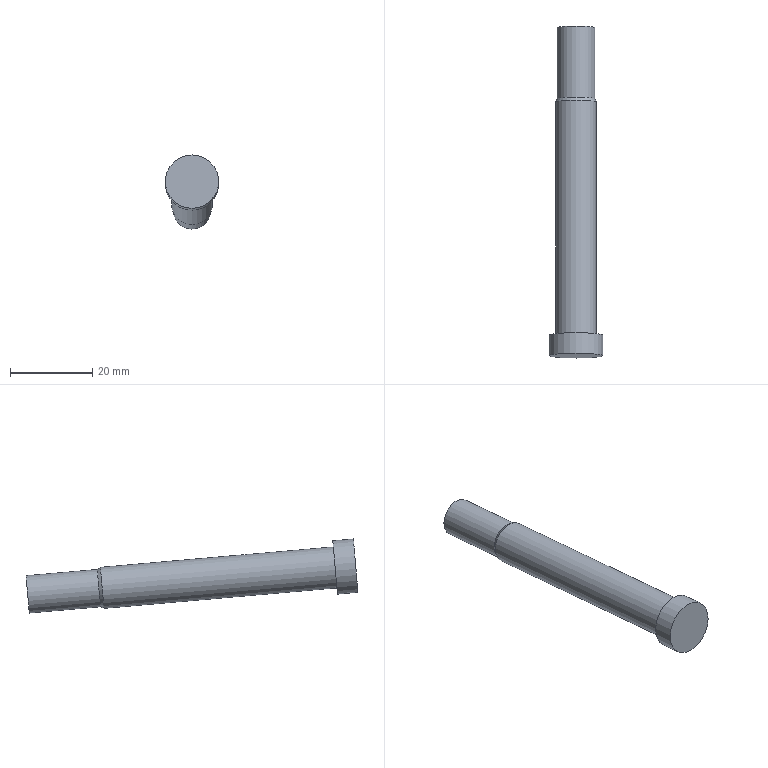Part | NX | features SPAS 10-80-7.100 2 | 1 solid | 7 faces | box 13 x 80.659 x 17.98 mm | volume 6314 mm3 | plane 3 | cylinder 3 | torus 1 | commonest cylinder face diameters 9.1 x1 10 x1 13 x1
STEP:
#1=CARTESIAN_POINT('',(-561.105,-62.517,-39.823));
#2=VERTEX_POINT('',#1);
#3=CARTESIAN_POINT('',(-561.105,-62.913,-44.355));
#4=DIRECTION('',(0.,0.9962,-0.08716));
#5=DIRECTION('',(0.,0.08716,0.9962));
#6=AXIS2_PLACEMENT_3D('',#3,#4,#5);
#7=CIRCLE('',#6,4.55);
#8=EDGE_CURVE('',#2,#2,#7,.F.);
#9=ORIENTED_EDGE('',*,*,#8,.F.);
#10=EDGE_LOOP('',(#9));
#11=FACE_BOUND('',#10,.T.);
#12=CARTESIAN_POINT('',(-561.105,-62.913,-44.355));
#13=DIRECTION('',(0.,0.9962,-0.08716));
#14=DIRECTION('',(0.,0.08716,0.9962));
#15=AXIS2_PLACEMENT_3D('',#12,#13,#14);
#16=PLANE('',#15);
#17=ADVANCED_FACE('',(#11),#16,.T.);
#18=CARTESIAN_POINT('',(-561.105,-79.809,-38.31));
#19=VERTEX_POINT('',#18);
#20=CARTESIAN_POINT('',(-561.105,-80.206,-42.843));
#21=DIRECTION('',(0.,0.9962,-0.08716));
#22=DIRECTION('',(0.,0.08716,0.9962));
#23=AXIS2_PLACEMENT_3D('',#20,#21,#22);
#24=CIRCLE('',#23,4.55);
#25=EDGE_CURVE('',#19,#19,#24,.T.);
#26=ORIENTED_EDGE('',*,*,#25,.T.);
#27=EDGE_LOOP('',(#26));
#28=FACE_BOUND('',#27,.T.);
#29=ORIENTED_EDGE('',*,*,#8,.T.);
#30=EDGE_LOOP('',(#29));
#31=FACE_BOUND('',#30,.T.);
#32=CARTESIAN_POINT('',(-561.105,-62.913,-44.355));
#33=DIRECTION('',(0.,-0.9962,0.08716));
#34=DIRECTION('',(0.,-0.08716,-0.9962));
#35=AXIS2_PLACEMENT_3D('',#32,#33,#34);
#36=CYLINDRICAL_SURFACE('',#35,4.55);
#37=ADVANCED_FACE('',(#28,#31),#36,.T.);
#38=CARTESIAN_POINT('',(-561.105,-137.192,-32.838));
#39=VERTEX_POINT('',#38);
#40=CARTESIAN_POINT('',(-561.105,-137.628,-37.819));
#41=DIRECTION('',(0.,0.9962,-0.08716));
#42=DIRECTION('',(0.,0.08716,0.9962));
#43=AXIS2_PLACEMENT_3D('',#40,#41,#42);
#44=CIRCLE('',#43,5.);
#45=EDGE_CURVE('',#39,#39,#44,.F.);
#46=ORIENTED_EDGE('',*,*,#45,.F.);
#47=EDGE_LOOP('',(#46));
#48=FACE_BOUND('',#47,.T.);
#49=CARTESIAN_POINT('',(-561.105,-81.466,-47.751));
#50=VERTEX_POINT('',#49);
#51=CARTESIAN_POINT('',(-561.105,-81.03,-42.77));
#52=DIRECTION('',(0.,-0.9962,0.08716));
#53=DIRECTION('',(0.,-0.08716,-0.9962));
#54=AXIS2_PLACEMENT_3D('',#51,#52,#53);
#55=CIRCLE('',#54,5.);
#56=EDGE_CURVE('',#50,#50,#55,.T.);
#57=ORIENTED_EDGE('',*,*,#56,.T.);
#58=EDGE_LOOP('',(#57));
#59=FACE_BOUND('',#58,.T.);
#60=CARTESIAN_POINT('',(-561.105,-81.03,-42.77));
#61=DIRECTION('',(0.,-0.9962,0.08716));
#62=DIRECTION('',(0.,-0.08716,-0.9962));
#63=AXIS2_PLACEMENT_3D('',#60,#61,#62);
#64=CYLINDRICAL_SURFACE('',#63,5.);
#65=ADVANCED_FACE('',(#48,#59),#64,.T.);
#66=CARTESIAN_POINT('',(-561.105,-142.042,-30.908));
#67=VERTEX_POINT('',#66);
#68=CARTESIAN_POINT('',(-561.105,-142.609,-37.383));
#69=DIRECTION('',(0.,0.9962,-0.08716));
#70=DIRECTION('',(0.,0.08716,0.9962));
#71=AXIS2_PLACEMENT_3D('',#68,#69,#70);
#72=CIRCLE('',#71,6.5);
#73=EDGE_CURVE('',#67,#67,#72,.T.);
#74=ORIENTED_EDGE('',*,*,#73,.F.);
#75=EDGE_LOOP('',(#74));
#76=FACE_BOUND('',#75,.T.);
#77=CARTESIAN_POINT('',(-561.105,-142.609,-37.383));
#78=DIRECTION('',(0.,-0.9962,0.08716));
#79=DIRECTION('',(0.,-0.08716,-0.9962));
#80=AXIS2_PLACEMENT_3D('',#77,#78,#79);
#81=PLANE('',#80);
#82=ADVANCED_FACE('',(#76),#81,.T.);
#83=ORIENTED_EDGE('',*,*,#45,.T.);
#84=EDGE_LOOP('',(#83));
#85=FACE_BOUND('',#84,.T.);
#86=CARTESIAN_POINT('',(-561.105,-138.194,-44.294));
#87=VERTEX_POINT('',#86);
#88=CARTESIAN_POINT('',(-561.105,-137.628,-37.819));
#89=DIRECTION('',(0.,-0.9962,0.08716));
#90=DIRECTION('',(0.,-0.08716,-0.9962));
#91=AXIS2_PLACEMENT_3D('',#88,#89,#90);
#92=CIRCLE('',#91,6.5);
#93=EDGE_CURVE('',#87,#87,#92,.T.);
#94=ORIENTED_EDGE('',*,*,#93,.F.);
#95=EDGE_LOOP('',(#94));
#96=FACE_BOUND('',#95,.T.);
#97=CARTESIAN_POINT('',(-561.105,-137.628,-37.819));
#98=DIRECTION('',(0.,0.9962,-0.08716));
#99=DIRECTION('',(0.,0.08716,0.9962));
#100=AXIS2_PLACEMENT_3D('',#97,#98,#99);
#101=PLANE('',#100);
#102=ADVANCED_FACE('',(#85,#96),#101,.T.);
#103=ORIENTED_EDGE('',*,*,#73,.T.);
#104=EDGE_LOOP('',(#103));
#105=FACE_BOUND('',#104,.T.);
#106=ORIENTED_EDGE('',*,*,#93,.T.);
#107=EDGE_LOOP('',(#106));
#108=FACE_BOUND('',#107,.T.);
#109=CARTESIAN_POINT('',(-561.105,-137.628,-37.819));
#110=DIRECTION('',(0.,-0.9962,0.08716));
#111=DIRECTION('',(0.,-0.08716,-0.9962));
#112=AXIS2_PLACEMENT_3D('',#109,#110,#111);
#113=CYLINDRICAL_SURFACE('',#112,6.5);
#114=ADVANCED_FACE('',(#105,#108),#113,.T.);
#115=ORIENTED_EDGE('',*,*,#25,.F.);
#116=EDGE_LOOP('',(#115));
#117=FACE_BOUND('',#116,.T.);
#118=ORIENTED_EDGE('',*,*,#56,.F.);
#119=EDGE_LOOP('',(#118));
#120=FACE_BOUND('',#119,.T.);
#121=CARTESIAN_POINT('',(-561.105,-75.864,-43.222));
#122=DIRECTION('',(0.,-0.9962,0.08716));
#123=DIRECTION('',(0.,-0.08716,-0.9962));
#124=AXIS2_PLACEMENT_3D('',#121,#122,#123);
#125=TOROIDAL_SURFACE('',#124,13.55,10.);
#126=ADVANCED_FACE('',(#117,#120),#125,.F.);
#127=CLOSED_SHELL('',(#17,#37,#65,#82,#102,#114,#126));
#128=MANIFOLD_SOLID_BREP('',#127);
#129=(LENGTH_UNIT()NAMED_UNIT(*)SI_UNIT(.MILLI.,.METRE.));
#130=UNCERTAINTY_MEASURE_WITH_UNIT(LENGTH_MEASURE(0.00001),#129,'','');
#131=(NAMED_UNIT(*)PLANE_ANGLE_UNIT()SI_UNIT($,.RADIAN.));
#132=(NAMED_UNIT(*)SI_UNIT($,.STERADIAN.)SOLID_ANGLE_UNIT());
#133=(GEOMETRIC_REPRESENTATION_CONTEXT(3)GLOBAL_UNCERTAINTY_ASSIGNED_CONTEXT((#130))GLOBAL_UNIT_ASSIGNED_CONTEXT((#129,#131,#132))REPRESENTATION_CONTEXT('',''));
#134=ADVANCED_BREP_SHAPE_REPRESENTATION('',(#128),#133);